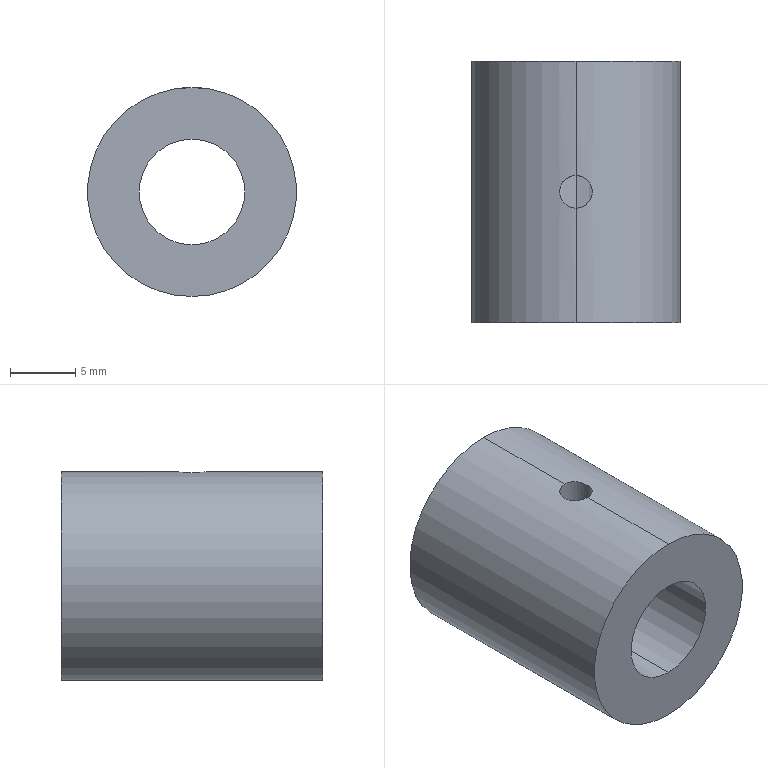Part | SolidWorks | features 3DProfileFeature 1, HoleWzd 1, Revolution 1 | 1 solid | 8 faces | box 16 x 20 x 16 mm | volume 2971 mm3 | cylinder 6 | plane 2 | commonest cylinder face diameters 2.5 x2 8.1 x2 16 x2
STEP:
#1=CARTESIAN_POINT('',(-1.25,20.516,3.852));
#2=VERTEX_POINT('',#1);
#3=CARTESIAN_POINT('',(0.,19.266,4.05));
#4=VERTEX_POINT('',#3);
#5=CARTESIAN_POINT('',(-1.25,20.516,3.852));
#6=CARTESIAN_POINT('',(-1.25,20.351,3.852));
#7=CARTESIAN_POINT('',(-1.217,20.187,3.863));
#8=CARTESIAN_POINT('',(-1.092,19.886,3.901));
#9=CARTESIAN_POINT('',(-0.9987,19.747,3.927));
#10=CARTESIAN_POINT('',(-0.7696,19.518,3.978));
#11=CARTESIAN_POINT('',(-0.6316,19.425,4.003));
#12=CARTESIAN_POINT('',(-0.33,19.299,4.039));
#13=CARTESIAN_POINT('',(-0.1662,19.266,4.05));
#14=CARTESIAN_POINT('',(0.,19.266,4.05));
#15=B_SPLINE_CURVE_WITH_KNOTS('',3,(#5,#6,#7,#8,#9,#10,#11,#12,#13,#14),.UNSPECIFIED.,.F.,.F.,(4,2,2,2,4),(0.005898,0.006389,0.006881,0.007372,0.007863),.UNSPECIFIED.);
#16=EDGE_CURVE('',#2,#4,#15,.T.);
#17=ORIENTED_EDGE('',*,*,#16,.F.);
#18=CARTESIAN_POINT('',(-1.25,20.516,7.902));
#19=VERTEX_POINT('',#18);
#20=CARTESIAN_POINT('',(-1.25,20.516,8.));
#21=DIRECTION('',(0.,0.,1.));
#22=VECTOR('',#21,1000.);
#23=LINE('',#20,#22);
#24=EDGE_CURVE('',#2,#19,#23,.T.);
#25=ORIENTED_EDGE('',*,*,#24,.T.);
#26=CARTESIAN_POINT('',(0.,19.266,8.));
#27=VERTEX_POINT('',#26);
#28=CARTESIAN_POINT('',(0.,19.266,8.));
#29=CARTESIAN_POINT('',(-0.1655,19.266,8.));
#30=CARTESIAN_POINT('',(-0.3279,19.299,7.995));
#31=CARTESIAN_POINT('',(-0.6306,19.424,7.977));
#32=CARTESIAN_POINT('',(-0.7691,19.517,7.964));
#33=CARTESIAN_POINT('',(-0.9994,19.748,7.938));
#34=CARTESIAN_POINT('',(-1.092,19.887,7.925));
#35=CARTESIAN_POINT('',(-1.217,20.188,7.907));
#36=CARTESIAN_POINT('',(-1.25,20.353,7.902));
#37=CARTESIAN_POINT('',(-1.25,20.516,7.902));
#38=B_SPLINE_CURVE_WITH_KNOTS('',3,(#28,#29,#30,#31,#32,#33,#34,#35,#36,#37),.UNSPECIFIED.,.F.,.F.,(4,2,2,2,4),(0.,0.0004894,0.0009788,0.001468,0.001958),.UNSPECIFIED.);
#39=EDGE_CURVE('',#27,#19,#38,.T.);
#40=ORIENTED_EDGE('',*,*,#39,.F.);
#41=CARTESIAN_POINT('',(1.25,20.516,7.902));
#42=VERTEX_POINT('',#41);
#43=CARTESIAN_POINT('',(1.25,20.516,7.902));
#44=CARTESIAN_POINT('',(1.25,20.351,7.902));
#45=CARTESIAN_POINT('',(1.217,20.188,7.907));
#46=CARTESIAN_POINT('',(1.092,19.886,7.925));
#47=CARTESIAN_POINT('',(0.9992,19.748,7.938));
#48=CARTESIAN_POINT('',(0.7692,19.518,7.964));
#49=CARTESIAN_POINT('',(0.6301,19.424,7.977));
#50=CARTESIAN_POINT('',(0.3296,19.299,7.995));
#51=CARTESIAN_POINT('',(0.1653,19.266,8.));
#52=CARTESIAN_POINT('',(0.,19.266,8.));
#53=B_SPLINE_CURVE_WITH_KNOTS('',3,(#43,#44,#45,#46,#47,#48,#49,#50,#51,#52),.UNSPECIFIED.,.F.,.F.,(4,2,2,2,4),(0.005871,0.00636,0.006849,0.007338,0.007827),.UNSPECIFIED.);
#54=EDGE_CURVE('',#42,#27,#53,.T.);
#55=ORIENTED_EDGE('',*,*,#54,.F.);
#56=CARTESIAN_POINT('',(1.25,20.516,3.852));
#57=VERTEX_POINT('',#56);
#58=CARTESIAN_POINT('',(1.25,20.516,8.));
#59=DIRECTION('',(0.,0.,1.));
#60=VECTOR('',#59,1000.);
#61=LINE('',#58,#60);
#62=EDGE_CURVE('',#57,#42,#61,.T.);
#63=ORIENTED_EDGE('',*,*,#62,.F.);
#64=CARTESIAN_POINT('',(0.,19.266,4.05));
#65=CARTESIAN_POINT('',(0.1663,19.266,4.05));
#66=CARTESIAN_POINT('',(0.3295,19.299,4.039));
#67=CARTESIAN_POINT('',(0.6319,19.425,4.003));
#68=CARTESIAN_POINT('',(0.7699,19.518,3.978));
#69=CARTESIAN_POINT('',(0.999,19.747,3.927));
#70=CARTESIAN_POINT('',(1.092,19.886,3.901));
#71=CARTESIAN_POINT('',(1.217,20.187,3.863));
#72=CARTESIAN_POINT('',(1.25,20.352,3.852));
#73=CARTESIAN_POINT('',(1.25,20.516,3.852));
#74=B_SPLINE_CURVE_WITH_KNOTS('',3,(#64,#65,#66,#67,#68,#69,#70,#71,#72,#73),.UNSPECIFIED.,.F.,.F.,(4,2,2,2,4),(0.,0.0004917,0.0009833,0.001475,0.001967),.UNSPECIFIED.);
#75=EDGE_CURVE('',#4,#57,#74,.T.);
#76=ORIENTED_EDGE('',*,*,#75,.F.);
#77=EDGE_LOOP('',(#17,#25,#40,#55,#63,#76));
#78=FACE_OUTER_BOUND('',#77,.T.);
#79=CARTESIAN_POINT('',(0.,20.516,8.));
#80=DIRECTION('',(0.,0.,1.));
#81=DIRECTION('',(1.,0.,0.));
#82=AXIS2_PLACEMENT_3D('',#79,#80,#81);
#83=CYLINDRICAL_SURFACE('',#82,1.25);
#84=ADVANCED_FACE('',(#78),#83,.F.);
#85=CARTESIAN_POINT('',(0.,10.516,-4.05));
#86=VERTEX_POINT('',#85);
#87=CARTESIAN_POINT('',(0.,10.516,4.05));
#88=VERTEX_POINT('',#87);
#89=CARTESIAN_POINT('',(0.,10.516,0.));
#90=DIRECTION('',(0.,1.,0.));
#91=DIRECTION('',(0.,0.,1.));
#92=AXIS2_PLACEMENT_3D('',#89,#90,#91);
#93=CIRCLE('',#92,4.05);
#94=EDGE_CURVE('',#86,#88,#93,.T.);
#95=ORIENTED_EDGE('',*,*,#94,.F.);
#96=CARTESIAN_POINT('',(0.,30.516,-4.05));
#97=VERTEX_POINT('',#96);
#98=CARTESIAN_POINT('',(0.,29.613,-4.05));
#99=DIRECTION('',(0.,1.,0.));
#100=VECTOR('',#99,1000.);
#101=LINE('',#98,#100);
#102=EDGE_CURVE('',#86,#97,#101,.T.);
#103=ORIENTED_EDGE('',*,*,#102,.T.);
#104=CARTESIAN_POINT('',(0.,30.516,4.05));
#105=VERTEX_POINT('',#104);
#106=CARTESIAN_POINT('',(0.,30.516,0.));
#107=DIRECTION('',(0.,1.,0.));
#108=DIRECTION('',(0.,0.,1.));
#109=AXIS2_PLACEMENT_3D('',#106,#107,#108);
#110=CIRCLE('',#109,4.05);
#111=EDGE_CURVE('',#97,#105,#110,.T.);
#112=ORIENTED_EDGE('',*,*,#111,.T.);
#113=CARTESIAN_POINT('',(0.,21.766,4.05));
#114=VERTEX_POINT('',#113);
#115=CARTESIAN_POINT('',(0.,29.613,4.05));
#116=DIRECTION('',(0.,1.,0.));
#117=VECTOR('',#116,1000.);
#118=LINE('',#115,#117);
#119=EDGE_CURVE('',#114,#105,#118,.T.);
#120=ORIENTED_EDGE('',*,*,#119,.F.);
#121=CARTESIAN_POINT('',(0.,21.766,4.05));
#122=CARTESIAN_POINT('',(-0.1638,21.766,4.05));
#123=CARTESIAN_POINT('',(-0.3292,21.733,4.039));
#124=CARTESIAN_POINT('',(-0.6306,21.608,4.003));
#125=CARTESIAN_POINT('',(-0.7685,21.515,3.978));
#126=CARTESIAN_POINT('',(-0.9992,21.285,3.927));
#127=CARTESIAN_POINT('',(-1.091,21.148,3.901));
#128=CARTESIAN_POINT('',(-1.186,20.92,3.873));
#129=CARTESIAN_POINT('',(-1.21,20.842,3.865));
#130=CARTESIAN_POINT('',(-1.242,20.682,3.855));
#131=CARTESIAN_POINT('',(-1.25,20.599,3.852));
#132=CARTESIAN_POINT('',(-1.25,20.516,3.852));
#133=B_SPLINE_CURVE_WITH_KNOTS('',3,(#121,#122,#123,#124,#125,#126,#127,#128,#129,#130,#131,#132),.UNSPECIFIED.,.F.,.F.,(4,2,2,2,2,4),(0.003932,0.004424,0.004915,0.005406,0.005652,0.005898),.UNSPECIFIED.);
#134=EDGE_CURVE('',#114,#2,#133,.T.);
#135=ORIENTED_EDGE('',*,*,#134,.T.);
#136=ORIENTED_EDGE('',*,*,#16,.T.);
#137=CARTESIAN_POINT('',(0.,29.613,4.05));
#138=DIRECTION('',(0.,1.,0.));
#139=VECTOR('',#138,1000.);
#140=LINE('',#137,#139);
#141=EDGE_CURVE('',#88,#4,#140,.T.);
#142=ORIENTED_EDGE('',*,*,#141,.F.);
#143=EDGE_LOOP('',(#95,#103,#112,#120,#135,#136,#142));
#144=FACE_OUTER_BOUND('',#143,.T.);
#145=CARTESIAN_POINT('',(0.,29.613,0.));
#146=DIRECTION('',(0.,1.,0.));
#147=DIRECTION('',(0.,0.,1.));
#148=AXIS2_PLACEMENT_3D('',#145,#146,#147);
#149=CYLINDRICAL_SURFACE('',#148,4.05);
#150=ADVANCED_FACE('',(#144),#149,.F.);
#151=CARTESIAN_POINT('',(0.,10.516,8.));
#152=VERTEX_POINT('',#151);
#153=CARTESIAN_POINT('',(0.,10.516,-8.));
#154=VERTEX_POINT('',#153);
#155=CARTESIAN_POINT('',(0.,10.516,0.));
#156=DIRECTION('',(0.,1.,0.));
#157=DIRECTION('',(0.,0.,1.));
#158=AXIS2_PLACEMENT_3D('',#155,#156,#157);
#159=CIRCLE('',#158,8.);
#160=EDGE_CURVE('',#152,#154,#159,.T.);
#161=ORIENTED_EDGE('',*,*,#160,.T.);
#162=CARTESIAN_POINT('',(0.,30.516,-8.));
#163=VERTEX_POINT('',#162);
#164=CARTESIAN_POINT('',(0.,29.613,-8.));
#165=DIRECTION('',(0.,1.,0.));
#166=VECTOR('',#165,1000.);
#167=LINE('',#164,#166);
#168=EDGE_CURVE('',#154,#163,#167,.T.);
#169=ORIENTED_EDGE('',*,*,#168,.T.);
#170=CARTESIAN_POINT('',(0.,30.516,8.));
#171=VERTEX_POINT('',#170);
#172=CARTESIAN_POINT('',(0.,30.516,0.));
#173=DIRECTION('',(0.,1.,0.));
#174=DIRECTION('',(0.,0.,1.));
#175=AXIS2_PLACEMENT_3D('',#172,#173,#174);
#176=CIRCLE('',#175,8.);
#177=EDGE_CURVE('',#171,#163,#176,.T.);
#178=ORIENTED_EDGE('',*,*,#177,.F.);
#179=CARTESIAN_POINT('',(0.,21.766,8.));
#180=VERTEX_POINT('',#179);
#181=CARTESIAN_POINT('',(0.,29.613,8.));
#182=DIRECTION('',(0.,1.,0.));
#183=VECTOR('',#182,1000.);
#184=LINE('',#181,#183);
#185=EDGE_CURVE('',#180,#171,#184,.T.);
#186=ORIENTED_EDGE('',*,*,#185,.F.);
#187=CARTESIAN_POINT('',(0.,21.766,8.));
#188=CARTESIAN_POINT('',(0.1633,21.766,8.));
#189=CARTESIAN_POINT('',(0.3281,21.733,7.995));
#190=CARTESIAN_POINT('',(0.6291,21.609,7.977));
#191=CARTESIAN_POINT('',(0.7683,21.516,7.964));
#192=CARTESIAN_POINT('',(0.9412,21.343,7.945));
#193=CARTESIAN_POINT('',(0.994,21.278,7.938));
#194=CARTESIAN_POINT('',(1.085,21.143,7.926));
#195=CARTESIAN_POINT('',(1.123,21.071,7.921));
#196=CARTESIAN_POINT('',(1.217,20.844,7.907));
#197=CARTESIAN_POINT('',(1.25,20.681,7.902));
#198=CARTESIAN_POINT('',(1.25,20.516,7.902));
#199=B_SPLINE_CURVE_WITH_KNOTS('',3,(#187,#188,#189,#190,#191,#192,#193,#194,#195,#196,#197,#198),.UNSPECIFIED.,.F.,.F.,(4,2,2,2,2,4),(0.003914,0.004403,0.004893,0.005137,0.005382,0.005871),.UNSPECIFIED.);
#200=EDGE_CURVE('',#180,#42,#199,.T.);
#201=ORIENTED_EDGE('',*,*,#200,.T.);
#202=ORIENTED_EDGE('',*,*,#54,.T.);
#203=CARTESIAN_POINT('',(0.,29.613,8.));
#204=DIRECTION('',(0.,1.,0.));
#205=VECTOR('',#204,1000.);
#206=LINE('',#203,#205);
#207=EDGE_CURVE('',#152,#27,#206,.T.);
#208=ORIENTED_EDGE('',*,*,#207,.F.);
#209=EDGE_LOOP('',(#161,#169,#178,#186,#201,#202,#208));
#210=FACE_OUTER_BOUND('',#209,.T.);
#211=CARTESIAN_POINT('',(0.,29.613,0.));
#212=DIRECTION('',(0.,1.,0.));
#213=DIRECTION('',(0.,0.,1.));
#214=AXIS2_PLACEMENT_3D('',#211,#212,#213);
#215=CYLINDRICAL_SURFACE('',#214,8.);
#216=ADVANCED_FACE('',(#210),#215,.T.);
#217=ORIENTED_EDGE('',*,*,#168,.F.);
#218=CARTESIAN_POINT('',(0.,10.516,0.));
#219=DIRECTION('',(0.,1.,0.));
#220=DIRECTION('',(0.,0.,1.));
#221=AXIS2_PLACEMENT_3D('',#218,#219,#220);
#222=CIRCLE('',#221,8.);
#223=EDGE_CURVE('',#154,#152,#222,.T.);
#224=ORIENTED_EDGE('',*,*,#223,.T.);
#225=ORIENTED_EDGE('',*,*,#207,.T.);
#226=ORIENTED_EDGE('',*,*,#39,.T.);
#227=CARTESIAN_POINT('',(-1.25,20.516,7.902));
#228=CARTESIAN_POINT('',(-1.25,20.598,7.902));
#229=CARTESIAN_POINT('',(-1.242,20.681,7.903));
#230=CARTESIAN_POINT('',(-1.21,20.841,7.908));
#231=CARTESIAN_POINT('',(-1.186,20.919,7.912));
#232=CARTESIAN_POINT('',(-1.092,21.146,7.925));
#233=CARTESIAN_POINT('',(-1.,21.284,7.938));
#234=CARTESIAN_POINT('',(-0.7673,21.517,7.964));
#235=CARTESIAN_POINT('',(-0.6297,21.608,7.977));
#236=CARTESIAN_POINT('',(-0.4029,21.702,7.99));
#237=CARTESIAN_POINT('',(-0.325,21.726,7.994));
#238=CARTESIAN_POINT('',(-0.1645,21.758,7.999));
#239=CARTESIAN_POINT('',(-0.08163,21.766,8.));
#240=CARTESIAN_POINT('',(0.,21.766,8.));
#241=B_SPLINE_CURVE_WITH_KNOTS('',3,(#227,#228,#229,#230,#231,#232,#233,#234,#235,#236,#237,#238,#239,#240),.UNSPECIFIED.,.F.,.F.,(4,2,2,2,2,2,4),(0.001958,0.002202,0.002447,0.002936,0.003425,0.003669,0.003914),.UNSPECIFIED.);
#242=EDGE_CURVE('',#19,#180,#241,.T.);
#243=ORIENTED_EDGE('',*,*,#242,.T.);
#244=ORIENTED_EDGE('',*,*,#185,.T.);
#245=CARTESIAN_POINT('',(0.,30.516,0.));
#246=DIRECTION('',(0.,1.,0.));
#247=DIRECTION('',(0.,0.,1.));
#248=AXIS2_PLACEMENT_3D('',#245,#246,#247);
#249=CIRCLE('',#248,8.);
#250=EDGE_CURVE('',#163,#171,#249,.T.);
#251=ORIENTED_EDGE('',*,*,#250,.F.);
#252=EDGE_LOOP('',(#217,#224,#225,#226,#243,#244,#251));
#253=FACE_OUTER_BOUND('',#252,.T.);
#254=CARTESIAN_POINT('',(0.,29.613,0.));
#255=DIRECTION('',(0.,1.,0.));
#256=DIRECTION('',(0.,0.,1.));
#257=AXIS2_PLACEMENT_3D('',#254,#255,#256);
#258=CYLINDRICAL_SURFACE('',#257,8.);
#259=ADVANCED_FACE('',(#253),#258,.T.);
#260=CARTESIAN_POINT('',(0.,30.516,0.));
#261=DIRECTION('',(0.,1.,0.));
#262=DIRECTION('',(0.,0.,1.));
#263=AXIS2_PLACEMENT_3D('',#260,#261,#262);
#264=CIRCLE('',#263,4.05);
#265=EDGE_CURVE('',#105,#97,#264,.T.);
#266=ORIENTED_EDGE('',*,*,#265,.F.);
#267=ORIENTED_EDGE('',*,*,#111,.F.);
#268=EDGE_LOOP('',(#266,#267));
#269=FACE_BOUND('',#268,.T.);
#270=ORIENTED_EDGE('',*,*,#177,.T.);
#271=ORIENTED_EDGE('',*,*,#250,.T.);
#272=EDGE_LOOP('',(#270,#271));
#273=FACE_OUTER_BOUND('',#272,.T.);
#274=CARTESIAN_POINT('',(4.05,30.516,0.));
#275=DIRECTION('',(0.,-1.,0.));
#276=DIRECTION('',(0.,0.,-1.));
#277=AXIS2_PLACEMENT_3D('',#274,#275,#276);
#278=PLANE('',#277);
#279=ADVANCED_FACE('',(#269,#273),#278,.F.);
#280=ORIENTED_EDGE('',*,*,#102,.F.);
#281=CARTESIAN_POINT('',(0.,10.516,0.));
#282=DIRECTION('',(0.,1.,0.));
#283=DIRECTION('',(0.,0.,1.));
#284=AXIS2_PLACEMENT_3D('',#281,#282,#283);
#285=CIRCLE('',#284,4.05);
#286=EDGE_CURVE('',#88,#86,#285,.T.);
#287=ORIENTED_EDGE('',*,*,#286,.F.);
#288=ORIENTED_EDGE('',*,*,#141,.T.);
#289=ORIENTED_EDGE('',*,*,#75,.T.);
#290=CARTESIAN_POINT('',(1.25,20.516,3.852));
#291=CARTESIAN_POINT('',(1.25,20.598,3.852));
#292=CARTESIAN_POINT('',(1.242,20.682,3.855));
#293=CARTESIAN_POINT('',(1.209,20.842,3.865));
#294=CARTESIAN_POINT('',(1.186,20.92,3.873));
#295=CARTESIAN_POINT('',(1.091,21.148,3.901));
#296=CARTESIAN_POINT('',(0.9987,21.285,3.927));
#297=CARTESIAN_POINT('',(0.8257,21.458,3.965));
#298=CARTESIAN_POINT('',(0.7631,21.509,3.978));
#299=CARTESIAN_POINT('',(0.6281,21.6,4.002));
#300=CARTESIAN_POINT('',(0.5549,21.639,4.013));
#301=CARTESIAN_POINT('',(0.329,21.733,4.039));
#302=CARTESIAN_POINT('',(0.1638,21.766,4.05));
#303=CARTESIAN_POINT('',(0.,21.766,4.05));
#304=B_SPLINE_CURVE_WITH_KNOTS('',3,(#290,#291,#292,#293,#294,#295,#296,#297,#298,#299,#300,#301,#302,#303),.UNSPECIFIED.,.F.,.F.,(4,2,2,2,2,2,4),(0.001967,0.002212,0.002458,0.002949,0.003195,0.003441,0.003932),.UNSPECIFIED.);
#305=EDGE_CURVE('',#57,#114,#304,.T.);
#306=ORIENTED_EDGE('',*,*,#305,.T.);
#307=ORIENTED_EDGE('',*,*,#119,.T.);
#308=ORIENTED_EDGE('',*,*,#265,.T.);
#309=EDGE_LOOP('',(#280,#287,#288,#289,#306,#307,#308));
#310=FACE_OUTER_BOUND('',#309,.T.);
#311=CARTESIAN_POINT('',(0.,29.613,0.));
#312=DIRECTION('',(0.,1.,0.));
#313=DIRECTION('',(0.,0.,1.));
#314=AXIS2_PLACEMENT_3D('',#311,#312,#313);
#315=CYLINDRICAL_SURFACE('',#314,4.05);
#316=ADVANCED_FACE('',(#310),#315,.F.);
#317=ORIENTED_EDGE('',*,*,#160,.F.);
#318=ORIENTED_EDGE('',*,*,#223,.F.);
#319=EDGE_LOOP('',(#317,#318));
#320=FACE_OUTER_BOUND('',#319,.T.);
#321=ORIENTED_EDGE('',*,*,#286,.T.);
#322=ORIENTED_EDGE('',*,*,#94,.T.);
#323=EDGE_LOOP('',(#321,#322));
#324=FACE_BOUND('',#323,.T.);
#325=CARTESIAN_POINT('',(4.05,10.516,0.));
#326=DIRECTION('',(0.,1.,0.));
#327=DIRECTION('',(0.,0.,1.));
#328=AXIS2_PLACEMENT_3D('',#325,#326,#327);
#329=PLANE('',#328);
#330=ADVANCED_FACE('',(#320,#324),#329,.F.);
#331=ORIENTED_EDGE('',*,*,#24,.F.);
#332=ORIENTED_EDGE('',*,*,#134,.F.);
#333=ORIENTED_EDGE('',*,*,#305,.F.);
#334=ORIENTED_EDGE('',*,*,#62,.T.);
#335=ORIENTED_EDGE('',*,*,#200,.F.);
#336=ORIENTED_EDGE('',*,*,#242,.F.);
#337=EDGE_LOOP('',(#331,#332,#333,#334,#335,#336));
#338=FACE_OUTER_BOUND('',#337,.T.);
#339=CARTESIAN_POINT('',(0.,20.516,8.));
#340=DIRECTION('',(0.,0.,1.));
#341=DIRECTION('',(1.,0.,0.));
#342=AXIS2_PLACEMENT_3D('',#339,#340,#341);
#343=CYLINDRICAL_SURFACE('',#342,1.25);
#344=ADVANCED_FACE('',(#338),#343,.F.);
#345=CLOSED_SHELL('',(#84,#150,#216,#259,#279,#316,#330,#344));
#346=MANIFOLD_SOLID_BREP('',#345);
#347=CARTESIAN_POINT('',(0.,0.,0.));
#348=DIRECTION('',(0.,0.,1.));
#349=DIRECTION('',(1.,0.,0.));
#350=AXIS2_PLACEMENT_3D('',#347,#348,#349);
#351=(LENGTH_UNIT()NAMED_UNIT(*)SI_UNIT(.MILLI.,.METRE.));
#352=UNCERTAINTY_MEASURE_WITH_UNIT(LENGTH_MEASURE(0.00001),#351,'','');
#353=(NAMED_UNIT(*)PLANE_ANGLE_UNIT()SI_UNIT($,.RADIAN.));
#354=(NAMED_UNIT(*)SI_UNIT($,.STERADIAN.)SOLID_ANGLE_UNIT());
#355=(GEOMETRIC_REPRESENTATION_CONTEXT(3)GLOBAL_UNCERTAINTY_ASSIGNED_CONTEXT((#352))GLOBAL_UNIT_ASSIGNED_CONTEXT((#351,#353,#354))REPRESENTATION_CONTEXT('',''));
#356=ADVANCED_BREP_SHAPE_REPRESENTATION('',(#346,#350),#355);